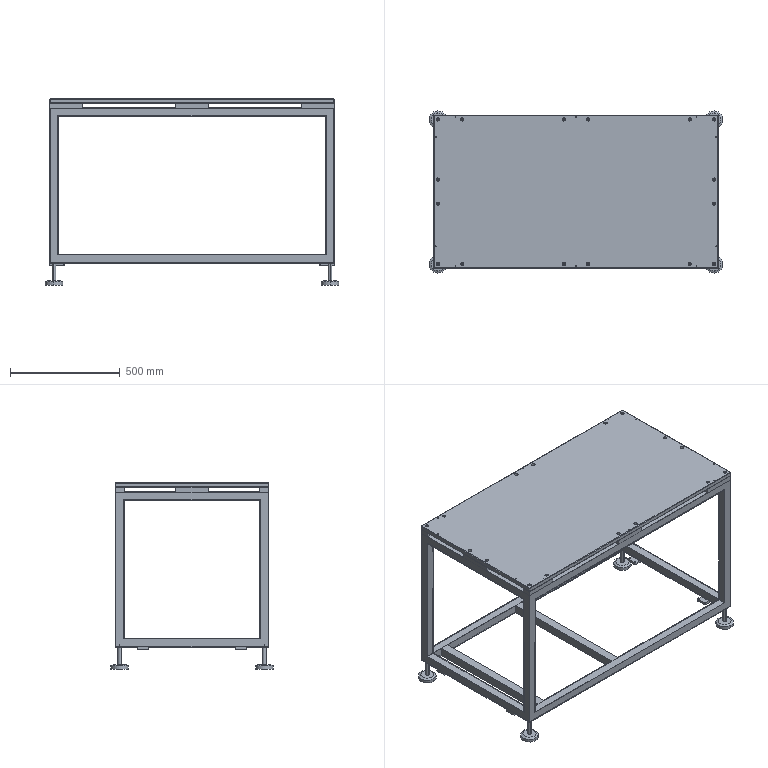Part | SolidWorks | 6 solids | 481 faces | box 1340 x 740 x 850 mm | volume 26625287 mm3 | plane 223 | cylinder 198 | cone 60 | commonest cylinder face diameters 4.2 x36 6.8 x36 5 x32 9 x32 15 x32 16 x16